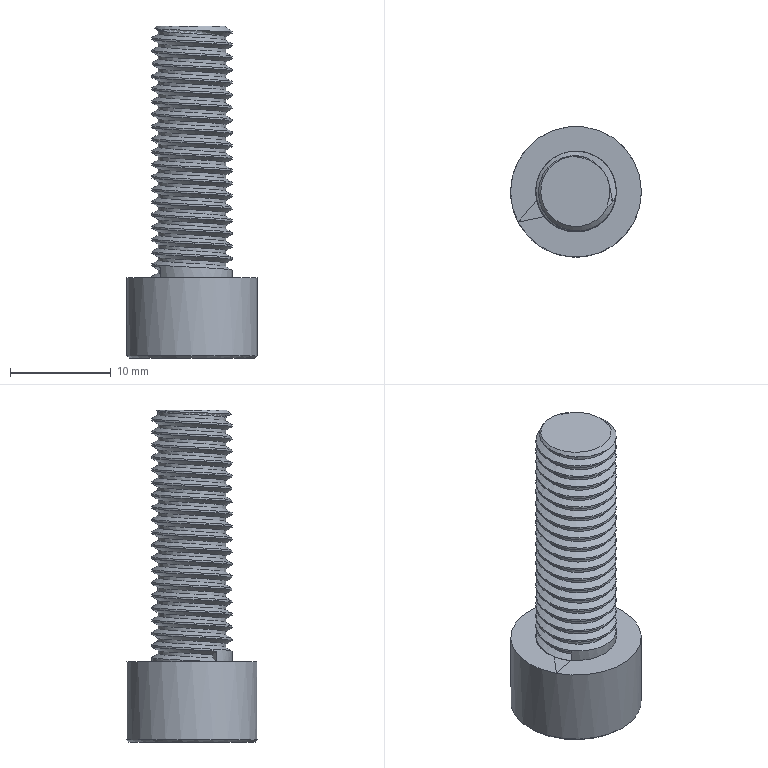Part | STEP file | Tube feed_id1690_x_t | 1 solid | 25 faces | box 13 x 13 x 33 mm | volume 1974 mm3 | plane 11 | cylinder 9 | spline 3 | torus 1 | cone 1 | commonest cylinder face diameters 0.4 x6 6.75 x1 8 x1 13 x1